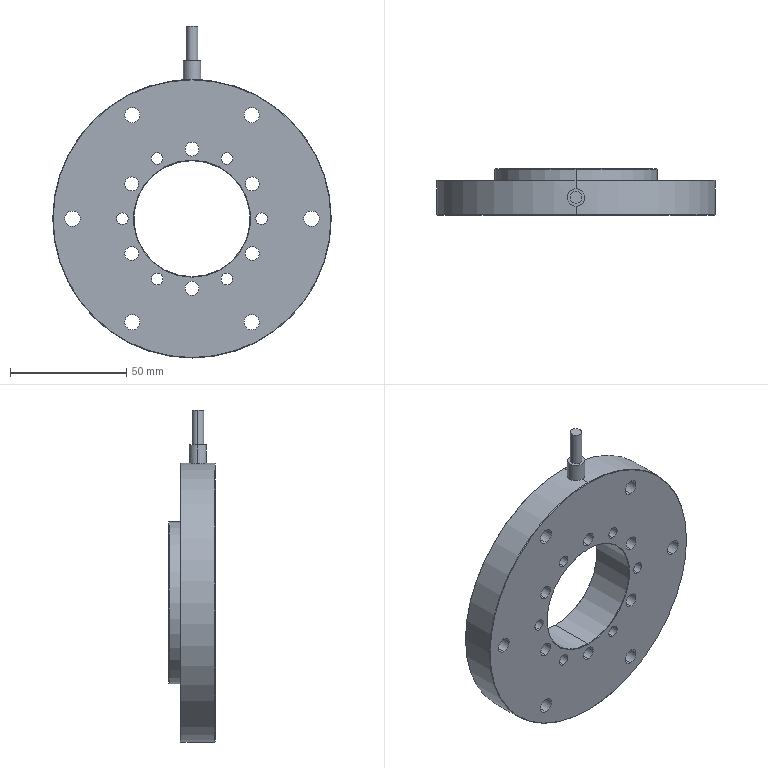Part | SolidWorks | features BaseBody 1 | 1 solid | 82 faces | box 120 x 20 x 143 mm | volume 136699 mm3 | cylinder 60 | plane 12 | cone 10 | commonest cylinder face diameters 5 x14 6 x12 6.6 x12 11 x12 7.5 x2 50 x2